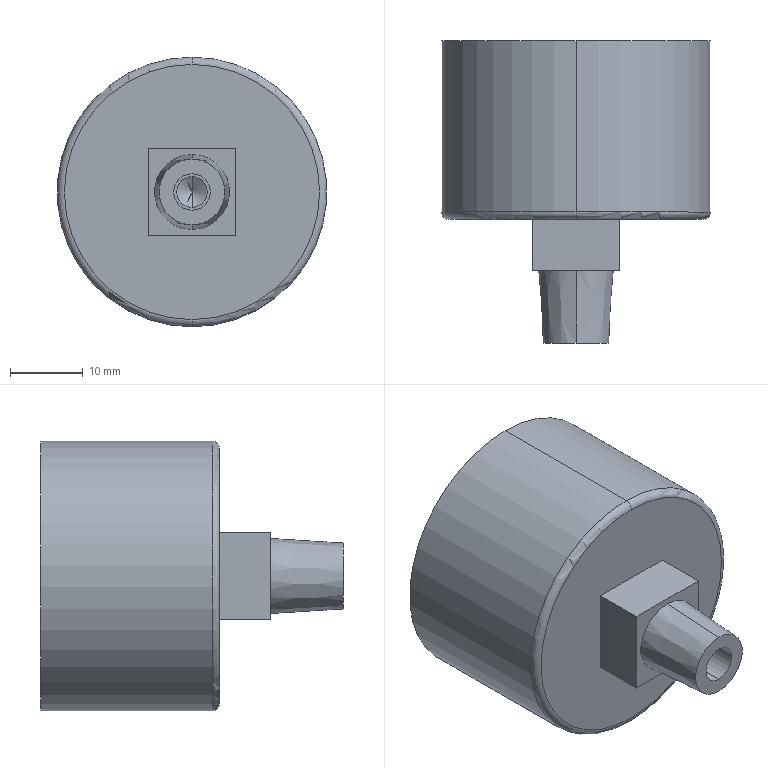Part | STEP file | VBA22A-03GN_G36-10-N01 | 1 solid | 21 faces | box 37 x 41.5 x 37 mm | volume 27826 mm3 | plane 9 | cylinder 6 | cone 4 | torus 2 | commonest cylinder face diameters 4.2 x2 5 x2 37 x2
STEP:
#1=CARTESIAN_POINT('',(0.,0.,0.));
#2=DIRECTION('',(0.,0.,1.));
#3=DIRECTION('',(1.,0.,0.));
#4=AXIS2_PLACEMENT_3D('',#1,#2,#3);
#5=CARTESIAN_POINT('',(0.,12.4,2.1));
#6=VERTEX_POINT('',#5);
#7=CARTESIAN_POINT('',(0.,12.4,-2.1));
#8=VERTEX_POINT('',#7);
#9=CARTESIAN_POINT('',(0.,12.4,0.));
#10=DIRECTION('',(0.,-1.,0.));
#11=DIRECTION('',(0.,0.,-1.));
#12=AXIS2_PLACEMENT_3D('',#9,#10,#11);
#13=CIRCLE('',#12,2.1);
#14=CARTESIAN_POINT('',(0.,12.4,0.));
#15=DIRECTION('',(0.,-1.,0.));
#16=DIRECTION('',(0.,0.,-1.));
#17=AXIS2_PLACEMENT_3D('',#14,#15,#16);
#18=CONICAL_SURFACE('',#17,2.1,1.03);
#19=CARTESIAN_POINT('',(0.,0.));
#20=DIRECTION('',(1.,0.));
#21=VECTOR('',#20,1.);
#22=LINE('',#19,#21);
#23=(GEOMETRIC_REPRESENTATION_CONTEXT(2)PARAMETRIC_REPRESENTATION_CONTEXT()REPRESENTATION_CONTEXT('',''));
#24=DEFINITIONAL_REPRESENTATION('',(#22),#23);
#25=PCURVE('',#18,#24);
#26=CARTESIAN_POINT('',(0.,0.,0.));
#27=DIRECTION('',(0.,-1.,0.));
#28=DIRECTION('',(0.,0.,-1.));
#29=AXIS2_PLACEMENT_3D('',#26,#27,#28);
#30=CYLINDRICAL_SURFACE('',#29,2.1);
#31=CARTESIAN_POINT('',(0.,-12.4));
#32=DIRECTION('',(1.,0.));
#33=VECTOR('',#32,1.);
#34=LINE('',#31,#33);
#35=(GEOMETRIC_REPRESENTATION_CONTEXT(2)PARAMETRIC_REPRESENTATION_CONTEXT()REPRESENTATION_CONTEXT('',''));
#36=DEFINITIONAL_REPRESENTATION('',(#34),#35);
#37=PCURVE('',#30,#36);
#38=SURFACE_CURVE('',#13,(#25,#37),.PCURVE_S1.);
#39=EDGE_CURVE('',#6,#8,#38,.T.);
#40=ORIENTED_EDGE('',*,*,#39,.F.);
#41=CARTESIAN_POINT('',(0.,13.662,0.));
#42=VERTEX_POINT('',#41);
#43=CARTESIAN_POINT('',(0.,12.4,2.1));
#44=DIRECTION('',(0.,-0.515,0.8572));
#45=VECTOR('',#44,1.);
#46=LINE('',#43,#45);
#47=CARTESIAN_POINT('',(3.142,0.));
#48=DIRECTION('',(0.,1.));
#49=VECTOR('',#48,1.);
#50=LINE('',#47,#49);
#51=(GEOMETRIC_REPRESENTATION_CONTEXT(2)PARAMETRIC_REPRESENTATION_CONTEXT()REPRESENTATION_CONTEXT('',''));
#52=DEFINITIONAL_REPRESENTATION('',(#50),#51);
#53=PCURVE('',#18,#52);
#54=CARTESIAN_POINT('',(0.,12.4,0.));
#55=DIRECTION('',(0.,-1.,0.));
#56=DIRECTION('',(0.,0.,-1.));
#57=AXIS2_PLACEMENT_3D('',#54,#55,#56);
#58=CONICAL_SURFACE('',#57,2.1,1.03);
#59=CARTESIAN_POINT('',(3.142,0.));
#60=DIRECTION('',(0.,1.));
#61=VECTOR('',#60,1.);
#62=LINE('',#59,#61);
#63=(GEOMETRIC_REPRESENTATION_CONTEXT(2)PARAMETRIC_REPRESENTATION_CONTEXT()REPRESENTATION_CONTEXT('',''));
#64=DEFINITIONAL_REPRESENTATION('',(#62),#63);
#65=PCURVE('',#58,#64);
#66=SURFACE_CURVE('',#46,(#53,#65),.PCURVE_S1.);
#67=EDGE_CURVE('',#42,#6,#66,.T.);
#68=ORIENTED_EDGE('',*,*,#67,.F.);
#69=CARTESIAN_POINT('',(0.,12.4,-2.1));
#70=DIRECTION('',(0.,-0.515,-0.8572));
#71=VECTOR('',#70,1.);
#72=LINE('',#69,#71);
#73=CARTESIAN_POINT('',(6.283,0.));
#74=DIRECTION('',(0.,1.));
#75=VECTOR('',#74,1.);
#76=LINE('',#73,#75);
#77=(GEOMETRIC_REPRESENTATION_CONTEXT(2)PARAMETRIC_REPRESENTATION_CONTEXT()REPRESENTATION_CONTEXT('',''));
#78=DEFINITIONAL_REPRESENTATION('',(#76),#77);
#79=PCURVE('',#18,#78);
#80=CARTESIAN_POINT('',(0.,0.));
#81=DIRECTION('',(0.,1.));
#82=VECTOR('',#81,1.);
#83=LINE('',#80,#82);
#84=(GEOMETRIC_REPRESENTATION_CONTEXT(2)PARAMETRIC_REPRESENTATION_CONTEXT()REPRESENTATION_CONTEXT('',''));
#85=DEFINITIONAL_REPRESENTATION('',(#83),#84);
#86=PCURVE('',#58,#85);
#87=SURFACE_CURVE('',#72,(#79,#86),.PCURVE_S1.);
#88=EDGE_CURVE('',#42,#8,#87,.T.);
#89=ORIENTED_EDGE('',*,*,#88,.T.);
#90=EDGE_LOOP('',(#40,#68,#89));
#91=FACE_BOUND('',#90,.F.);
#92=ADVANCED_FACE('',(#91),#18,.F.);
#93=CARTESIAN_POINT('',(0.,10.,-2.1));
#94=VERTEX_POINT('',#93);
#95=CARTESIAN_POINT('',(0.,0.,-2.1));
#96=DIRECTION('',(0.,-1.,0.));
#97=VECTOR('',#96,1.);
#98=LINE('',#95,#97);
#99=CARTESIAN_POINT('',(6.283,0.));
#100=DIRECTION('',(0.,1.));
#101=VECTOR('',#100,1.);
#102=LINE('',#99,#101);
#103=(GEOMETRIC_REPRESENTATION_CONTEXT(2)PARAMETRIC_REPRESENTATION_CONTEXT()REPRESENTATION_CONTEXT('',''));
#104=DEFINITIONAL_REPRESENTATION('',(#102),#103);
#105=PCURVE('',#30,#104);
#106=CARTESIAN_POINT('',(0.,0.,0.));
#107=DIRECTION('',(0.,-1.,0.));
#108=DIRECTION('',(0.,0.,-1.));
#109=AXIS2_PLACEMENT_3D('',#106,#107,#108);
#110=CYLINDRICAL_SURFACE('',#109,2.1);
#111=CARTESIAN_POINT('',(0.,0.));
#112=DIRECTION('',(0.,1.));
#113=VECTOR('',#112,1.);
#114=LINE('',#111,#113);
#115=(GEOMETRIC_REPRESENTATION_CONTEXT(2)PARAMETRIC_REPRESENTATION_CONTEXT()REPRESENTATION_CONTEXT('',''));
#116=DEFINITIONAL_REPRESENTATION('',(#114),#115);
#117=PCURVE('',#110,#116);
#118=SURFACE_CURVE('',#98,(#105,#117),.PCURVE_S1.);
#119=EDGE_CURVE('',#8,#94,#118,.T.);
#120=ORIENTED_EDGE('',*,*,#119,.T.);
#121=CARTESIAN_POINT('',(0.,10.,2.1));
#122=VERTEX_POINT('',#121);
#123=CARTESIAN_POINT('',(0.,10.,0.));
#124=DIRECTION('',(0.,-1.,0.));
#125=DIRECTION('',(0.,0.,-1.));
#126=AXIS2_PLACEMENT_3D('',#123,#124,#125);
#127=CIRCLE('',#126,2.1);
#128=CARTESIAN_POINT('',(0.,-10.));
#129=DIRECTION('',(1.,0.));
#130=VECTOR('',#129,1.);
#131=LINE('',#128,#130);
#132=(GEOMETRIC_REPRESENTATION_CONTEXT(2)PARAMETRIC_REPRESENTATION_CONTEXT()REPRESENTATION_CONTEXT('',''));
#133=DEFINITIONAL_REPRESENTATION('',(#131),#132);
#134=PCURVE('',#30,#133);
#135=CARTESIAN_POINT('',(2.1,10.,0.));
#136=DIRECTION('',(0.,1.,0.));
#137=DIRECTION('',(0.,0.,1.));
#138=AXIS2_PLACEMENT_3D('',#135,#136,#137);
#139=PLANE('',#138);
#140=CARTESIAN_POINT('',(-2.1,-2.1));
#141=CARTESIAN_POINT('',(-2.1,1.537));
#142=CARTESIAN_POINT('',(1.05,-0.2813));
#143=CARTESIAN_POINT('',(4.2,-2.1));
#144=CARTESIAN_POINT('',(1.05,-3.919));
#145=CARTESIAN_POINT('',(-2.1,-5.737));
#146=CARTESIAN_POINT('',(-2.1,-2.1));
#147=(BOUNDED_CURVE()B_SPLINE_CURVE(2,(#140,#141,#142,#143,#144,#145,#146),.UNSPECIFIED.,.T.,.F.)B_SPLINE_CURVE_WITH_KNOTS((1,2,2,2,2,1),(-2.094,0.,2.094,4.189,6.283,8.378),.UNSPECIFIED.)CURVE()GEOMETRIC_REPRESENTATION_ITEM()RATIONAL_B_SPLINE_CURVE((1.,0.5,1.,0.5,1.,0.5,1.))REPRESENTATION_ITEM(''));
#148=(GEOMETRIC_REPRESENTATION_CONTEXT(2)PARAMETRIC_REPRESENTATION_CONTEXT()REPRESENTATION_CONTEXT('',''));
#149=DEFINITIONAL_REPRESENTATION('',(#147),#148);
#150=PCURVE('',#139,#149);
#151=SURFACE_CURVE('',#127,(#134,#150),.PCURVE_S1.);
#152=EDGE_CURVE('',#122,#94,#151,.T.);
#153=ORIENTED_EDGE('',*,*,#152,.F.);
#154=CARTESIAN_POINT('',(0.,0.,2.1));
#155=DIRECTION('',(0.,-1.,0.));
#156=VECTOR('',#155,1.);
#157=LINE('',#154,#156);
#158=CARTESIAN_POINT('',(3.142,0.));
#159=DIRECTION('',(0.,1.));
#160=VECTOR('',#159,1.);
#161=LINE('',#158,#160);
#162=(GEOMETRIC_REPRESENTATION_CONTEXT(2)PARAMETRIC_REPRESENTATION_CONTEXT()REPRESENTATION_CONTEXT('',''));
#163=DEFINITIONAL_REPRESENTATION('',(#161),#162);
#164=PCURVE('',#30,#163);
#165=CARTESIAN_POINT('',(3.142,0.));
#166=DIRECTION('',(0.,1.));
#167=VECTOR('',#166,1.);
#168=LINE('',#165,#167);
#169=(GEOMETRIC_REPRESENTATION_CONTEXT(2)PARAMETRIC_REPRESENTATION_CONTEXT()REPRESENTATION_CONTEXT('',''));
#170=DEFINITIONAL_REPRESENTATION('',(#168),#169);
#171=PCURVE('',#110,#170);
#172=SURFACE_CURVE('',#157,(#164,#171),.PCURVE_S1.);
#173=EDGE_CURVE('',#6,#122,#172,.T.);
#174=ORIENTED_EDGE('',*,*,#173,.F.);
#175=ORIENTED_EDGE('',*,*,#39,.T.);
#176=EDGE_LOOP('',(#120,#153,#174,#175));
#177=FACE_BOUND('',#176,.F.);
#178=ADVANCED_FACE('',(#177),#30,.F.);
#179=CARTESIAN_POINT('',(0.,10.,-2.5));
#180=VERTEX_POINT('',#179);
#181=CARTESIAN_POINT('',(0.,0.,-2.5));
#182=VERTEX_POINT('',#181);
#183=CARTESIAN_POINT('',(0.,0.,-2.5));
#184=DIRECTION('',(0.,-1.,0.));
#185=VECTOR('',#184,1.);
#186=LINE('',#183,#185);
#187=CARTESIAN_POINT('',(0.,0.,0.));
#188=DIRECTION('',(0.,-1.,0.));
#189=DIRECTION('',(0.,0.,-1.));
#190=AXIS2_PLACEMENT_3D('',#187,#188,#189);
#191=CYLINDRICAL_SURFACE('',#190,2.5);
#192=CARTESIAN_POINT('',(6.283,0.));
#193=DIRECTION('',(0.,1.));
#194=VECTOR('',#193,1.);
#195=LINE('',#192,#194);
#196=(GEOMETRIC_REPRESENTATION_CONTEXT(2)PARAMETRIC_REPRESENTATION_CONTEXT()REPRESENTATION_CONTEXT('',''));
#197=DEFINITIONAL_REPRESENTATION('',(#195),#196);
#198=PCURVE('',#191,#197);
#199=CARTESIAN_POINT('',(0.,0.,0.));
#200=DIRECTION('',(0.,-1.,0.));
#201=DIRECTION('',(0.,0.,-1.));
#202=AXIS2_PLACEMENT_3D('',#199,#200,#201);
#203=CYLINDRICAL_SURFACE('',#202,2.5);
#204=CARTESIAN_POINT('',(0.,0.));
#205=DIRECTION('',(0.,1.));
#206=VECTOR('',#205,1.);
#207=LINE('',#204,#206);
#208=(GEOMETRIC_REPRESENTATION_CONTEXT(2)PARAMETRIC_REPRESENTATION_CONTEXT()REPRESENTATION_CONTEXT('',''));
#209=DEFINITIONAL_REPRESENTATION('',(#207),#208);
#210=PCURVE('',#203,#209);
#211=SURFACE_CURVE('',#186,(#198,#210),.PCURVE_S1.);
#212=EDGE_CURVE('',#180,#182,#211,.T.);
#213=ORIENTED_EDGE('',*,*,#212,.T.);
#214=CARTESIAN_POINT('',(0.,0.,2.5));
#215=VERTEX_POINT('',#214);
#216=CARTESIAN_POINT('',(0.,0.,0.));
#217=DIRECTION('',(0.,-1.,0.));
#218=DIRECTION('',(0.,0.,-1.));
#219=AXIS2_PLACEMENT_3D('',#216,#217,#218);
#220=CIRCLE('',#219,2.5);
#221=CARTESIAN_POINT('',(0.,0.));
#222=DIRECTION('',(1.,0.));
#223=VECTOR('',#222,1.);
#224=LINE('',#221,#223);
#225=(GEOMETRIC_REPRESENTATION_CONTEXT(2)PARAMETRIC_REPRESENTATION_CONTEXT()REPRESENTATION_CONTEXT('',''));
#226=DEFINITIONAL_REPRESENTATION('',(#224),#225);
#227=PCURVE('',#191,#226);
#228=CARTESIAN_POINT('',(0.,0.,0.));
#229=DIRECTION('',(0.,-1.,0.));
#230=DIRECTION('',(0.,0.,-1.));
#231=AXIS2_PLACEMENT_3D('',#228,#229,#230);
#232=PLANE('',#231);
#233=CARTESIAN_POINT('',(0.,0.));
#234=DIRECTION('',(1.,0.));
#235=AXIS2_PLACEMENT_2D('',#233,#234);
#236=CIRCLE('',#235,2.5);
#237=(GEOMETRIC_REPRESENTATION_CONTEXT(2)PARAMETRIC_REPRESENTATION_CONTEXT()REPRESENTATION_CONTEXT('',''));
#238=DEFINITIONAL_REPRESENTATION('',(#236),#237);
#239=PCURVE('',#232,#238);
#240=SURFACE_CURVE('',#220,(#227,#239),.PCURVE_S1.);
#241=EDGE_CURVE('',#215,#182,#240,.T.);
#242=ORIENTED_EDGE('',*,*,#241,.F.);
#243=CARTESIAN_POINT('',(0.,10.,2.5));
#244=VERTEX_POINT('',#243);
#245=CARTESIAN_POINT('',(0.,0.,2.5));
#246=DIRECTION('',(0.,-1.,0.));
#247=VECTOR('',#246,1.);
#248=LINE('',#245,#247);
#249=CARTESIAN_POINT('',(3.142,0.));
#250=DIRECTION('',(0.,1.));
#251=VECTOR('',#250,1.);
#252=LINE('',#249,#251);
#253=(GEOMETRIC_REPRESENTATION_CONTEXT(2)PARAMETRIC_REPRESENTATION_CONTEXT()REPRESENTATION_CONTEXT('',''));
#254=DEFINITIONAL_REPRESENTATION('',(#252),#253);
#255=PCURVE('',#191,#254);
#256=CARTESIAN_POINT('',(3.142,0.));
#257=DIRECTION('',(0.,1.));
#258=VECTOR('',#257,1.);
#259=LINE('',#256,#258);
#260=(GEOMETRIC_REPRESENTATION_CONTEXT(2)PARAMETRIC_REPRESENTATION_CONTEXT()REPRESENTATION_CONTEXT('',''));
#261=DEFINITIONAL_REPRESENTATION('',(#259),#260);
#262=PCURVE('',#203,#261);
#263=SURFACE_CURVE('',#248,(#255,#262),.PCURVE_S1.);
#264=EDGE_CURVE('',#244,#215,#263,.T.);
#265=ORIENTED_EDGE('',*,*,#264,.F.);
#266=CARTESIAN_POINT('',(0.,10.,0.));
#267=DIRECTION('',(0.,-1.,0.));
#268=DIRECTION('',(0.,0.,-1.));
#269=AXIS2_PLACEMENT_3D('',#266,#267,#268);
#270=CIRCLE('',#269,2.5);
#271=CARTESIAN_POINT('',(0.,-10.));
#272=DIRECTION('',(1.,0.));
#273=VECTOR('',#272,1.);
#274=LINE('',#271,#273);
#275=(GEOMETRIC_REPRESENTATION_CONTEXT(2)PARAMETRIC_REPRESENTATION_CONTEXT()REPRESENTATION_CONTEXT('',''));
#276=DEFINITIONAL_REPRESENTATION('',(#274),#275);
#277=PCURVE('',#191,#276);
#278=CARTESIAN_POINT('',(-2.5,-2.1));
#279=CARTESIAN_POINT('',(-2.5,2.23));
#280=CARTESIAN_POINT('',(1.25,0.06506));
#281=CARTESIAN_POINT('',(5.,-2.1));
#282=CARTESIAN_POINT('',(1.25,-4.265));
#283=CARTESIAN_POINT('',(-2.5,-6.43));
#284=CARTESIAN_POINT('',(-2.5,-2.1));
#285=(BOUNDED_CURVE()B_SPLINE_CURVE(2,(#278,#279,#280,#281,#282,#283,#284),.UNSPECIFIED.,.T.,.F.)B_SPLINE_CURVE_WITH_KNOTS((1,2,2,2,2,1),(-2.094,0.,2.094,4.189,6.283,8.378),.UNSPECIFIED.)CURVE()GEOMETRIC_REPRESENTATION_ITEM()RATIONAL_B_SPLINE_CURVE((1.,0.5,1.,0.5,1.,0.5,1.))REPRESENTATION_ITEM(''));
#286=(GEOMETRIC_REPRESENTATION_CONTEXT(2)PARAMETRIC_REPRESENTATION_CONTEXT()REPRESENTATION_CONTEXT('',''));
#287=DEFINITIONAL_REPRESENTATION('',(#285),#286);
#288=PCURVE('',#139,#287);
#289=SURFACE_CURVE('',#270,(#277,#288),.PCURVE_S1.);
#290=EDGE_CURVE('',#244,#180,#289,.T.);
#291=ORIENTED_EDGE('',*,*,#290,.T.);
#292=EDGE_LOOP('',(#213,#242,#265,#291));
#293=FACE_BOUND('',#292,.F.);
#294=ADVANCED_FACE('',(#293),#191,.F.);
#295=CARTESIAN_POINT('',(0.,0.,-4.521));
#296=VERTEX_POINT('',#295);
#297=CARTESIAN_POINT('',(0.,0.,4.521));
#298=VERTEX_POINT('',#297);
#299=CARTESIAN_POINT('',(0.,0.,0.));
#300=DIRECTION('',(0.,-1.,0.));
#301=DIRECTION('',(0.,0.,-1.));
#302=AXIS2_PLACEMENT_3D('',#299,#300,#301);
#303=CIRCLE('',#302,4.521);
#304=CARTESIAN_POINT('',(0.,0.,0.));
#305=DIRECTION('',(0.,1.,0.));
#306=DIRECTION('',(0.,0.,1.));
#307=AXIS2_PLACEMENT_3D('',#304,#305,#306);
#308=CONICAL_SURFACE('',#307,4.521,0.06283);
#309=CARTESIAN_POINT('',(3.142,0.));
#310=DIRECTION('',(-1.,0.));
#311=VECTOR('',#310,1.);
#312=LINE('',#309,#311);
#313=(GEOMETRIC_REPRESENTATION_CONTEXT(2)PARAMETRIC_REPRESENTATION_CONTEXT()REPRESENTATION_CONTEXT('',''));
#314=DEFINITIONAL_REPRESENTATION('',(#312),#313);
#315=PCURVE('',#308,#314);
#316=CARTESIAN_POINT('',(0.,0.));
#317=DIRECTION('',(1.,0.));
#318=AXIS2_PLACEMENT_2D('',#316,#317);
#319=CIRCLE('',#318,4.521);
#320=(GEOMETRIC_REPRESENTATION_CONTEXT(2)PARAMETRIC_REPRESENTATION_CONTEXT()REPRESENTATION_CONTEXT('',''));
#321=DEFINITIONAL_REPRESENTATION('',(#319),#320);
#322=PCURVE('',#232,#321);
#323=SURFACE_CURVE('',#303,(#315,#322),.PCURVE_S1.);
#324=EDGE_CURVE('',#296,#298,#323,.T.);
#325=ORIENTED_EDGE('',*,*,#324,.F.);
#326=CARTESIAN_POINT('',(0.,10.,-5.15));
#327=VERTEX_POINT('',#326);
#328=CARTESIAN_POINT('',(0.,0.,-4.521));
#329=DIRECTION('',(0.,0.998,-0.06279));
#330=VECTOR('',#329,1.);
#331=LINE('',#328,#330);
#332=CARTESIAN_POINT('',(3.142,0.));
#333=DIRECTION('',(0.,1.));
#334=VECTOR('',#333,1.);
#335=LINE('',#332,#334);
#336=(GEOMETRIC_REPRESENTATION_CONTEXT(2)PARAMETRIC_REPRESENTATION_CONTEXT()REPRESENTATION_CONTEXT('',''));
#337=DEFINITIONAL_REPRESENTATION('',(#335),#336);
#338=PCURVE('',#308,#337);
#339=CARTESIAN_POINT('',(0.,0.,0.));
#340=DIRECTION('',(0.,1.,0.));
#341=DIRECTION('',(0.,0.,1.));
#342=AXIS2_PLACEMENT_3D('',#339,#340,#341);
#343=CONICAL_SURFACE('',#342,4.521,0.06283);
#344=CARTESIAN_POINT('',(3.142,0.));
#345=DIRECTION('',(0.,1.));
#346=VECTOR('',#345,1.);
#347=LINE('',#344,#346);
#348=(GEOMETRIC_REPRESENTATION_CONTEXT(2)PARAMETRIC_REPRESENTATION_CONTEXT()REPRESENTATION_CONTEXT('',''));
#349=DEFINITIONAL_REPRESENTATION('',(#347),#348);
#350=PCURVE('',#343,#349);
#351=SURFACE_CURVE('',#331,(#338,#350),.PCURVE_S1.);
#352=EDGE_CURVE('',#296,#327,#351,.T.);
#353=ORIENTED_EDGE('',*,*,#352,.T.);
#354=CARTESIAN_POINT('',(0.,10.,5.15));
#355=VERTEX_POINT('',#354);
#356=CARTESIAN_POINT('',(0.,10.,0.));
#357=DIRECTION('',(0.,-1.,0.));
#358=DIRECTION('',(0.,0.,1.));
#359=AXIS2_PLACEMENT_3D('',#356,#357,#358);
#360=CIRCLE('',#359,5.15);
#361=CARTESIAN_POINT('',(6.283,10.));
#362=DIRECTION('',(-1.,0.));
#363=VECTOR('',#362,1.);
#364=LINE('',#361,#363);
#365=(GEOMETRIC_REPRESENTATION_CONTEXT(2)PARAMETRIC_REPRESENTATION_CONTEXT()REPRESENTATION_CONTEXT('',''));
#366=DEFINITIONAL_REPRESENTATION('',(#364),#365);
#367=PCURVE('',#308,#366);
#368=CARTESIAN_POINT('',(-6.,10.,6.));
#369=DIRECTION('',(0.,1.,0.));
#370=DIRECTION('',(0.,0.,1.));
#371=AXIS2_PLACEMENT_3D('',#368,#369,#370);
#372=PLANE('',#371);
#373=CARTESIAN_POINT('',(-0.85,6.));
#374=CARTESIAN_POINT('',(-0.85,-2.92));
#375=CARTESIAN_POINT('',(-8.575,1.54));
#376=CARTESIAN_POINT('',(-16.3,6.));
#377=CARTESIAN_POINT('',(-8.575,10.46));
#378=CARTESIAN_POINT('',(-0.85,14.92));
#379=CARTESIAN_POINT('',(-0.85,6.));
#380=(BOUNDED_CURVE()B_SPLINE_CURVE(2,(#373,#374,#375,#376,#377,#378,#379),.UNSPECIFIED.,.T.,.F.)B_SPLINE_CURVE_WITH_KNOTS((1,2,2,2,2,1),(-2.094,0.,2.094,4.189,6.283,8.378),.UNSPECIFIED.)CURVE()GEOMETRIC_REPRESENTATION_ITEM()RATIONAL_B_SPLINE_CURVE((1.,0.5,1.,0.5,1.,0.5,1.))REPRESENTATION_ITEM(''));
#381=(GEOMETRIC_REPRESENTATION_CONTEXT(2)PARAMETRIC_REPRESENTATION_CONTEXT()REPRESENTATION_CONTEXT('',''));
#382=DEFINITIONAL_REPRESENTATION('',(#380),#381);
#383=PCURVE('',#372,#382);
#384=SURFACE_CURVE('',#360,(#367,#383),.PCURVE_S1.);
#385=EDGE_CURVE('',#327,#355,#384,.T.);
#386=ORIENTED_EDGE('',*,*,#385,.T.);
#387=CARTESIAN_POINT('',(0.,0.,4.521));
#388=DIRECTION('',(0.,0.998,0.06279));
#389=VECTOR('',#388,1.);
#390=LINE('',#387,#389);
#391=CARTESIAN_POINT('',(0.,0.));
#392=DIRECTION('',(0.,1.));
#393=VECTOR('',#392,1.);
#394=LINE('',#391,#393);
#395=(GEOMETRIC_REPRESENTATION_CONTEXT(2)PARAMETRIC_REPRESENTATION_CONTEXT()REPRESENTATION_CONTEXT('',''));
#396=DEFINITIONAL_REPRESENTATION('',(#394),#395);
#397=PCURVE('',#308,#396);
#398=CARTESIAN_POINT('',(6.283,0.));
#399=DIRECTION('',(0.,1.));
#400=VECTOR('',#399,1.);
#401=LINE('',#398,#400);
#402=(GEOMETRIC_REPRESENTATION_CONTEXT(2)PARAMETRIC_REPRESENTATION_CONTEXT()REPRESENTATION_CONTEXT('',''));
#403=DEFINITIONAL_REPRESENTATION('',(#401),#402);
#404=PCURVE('',#343,#403);
#405=SURFACE_CURVE('',#390,(#397,#404),.PCURVE_S1.);
#406=EDGE_CURVE('',#298,#355,#405,.T.);
#407=ORIENTED_EDGE('',*,*,#406,.F.);
#408=EDGE_LOOP('',(#325,#353,#386,#407));
#409=FACE_BOUND('',#408,.T.);
#410=ADVANCED_FACE('',(#409),#308,.T.);
#411=CARTESIAN_POINT('',(0.,41.5,-18.5));
#412=VERTEX_POINT('',#411);
#413=CARTESIAN_POINT('',(0.,41.5,18.5));
#414=VERTEX_POINT('',#413);
#415=CARTESIAN_POINT('',(0.,41.5,0.));
#416=DIRECTION('',(0.,-1.,0.));
#417=DIRECTION('',(0.,0.,-1.));
#418=AXIS2_PLACEMENT_3D('',#415,#416,#417);
#419=CIRCLE('',#418,18.5);
#420=CARTESIAN_POINT('',(0.,0.,0.));
#421=DIRECTION('',(0.,-1.,0.));
#422=DIRECTION('',(0.,0.,-1.));
#423=AXIS2_PLACEMENT_3D('',#420,#421,#422);
#424=CYLINDRICAL_SURFACE('',#423,18.5);
#425=CARTESIAN_POINT('',(0.,-41.5));
#426=DIRECTION('',(1.,0.));
#427=VECTOR('',#426,1.);
#428=LINE('',#425,#427);
#429=(GEOMETRIC_REPRESENTATION_CONTEXT(2)PARAMETRIC_REPRESENTATION_CONTEXT()REPRESENTATION_CONTEXT('',''));
#430=DEFINITIONAL_REPRESENTATION('',(#428),#429);
#431=PCURVE('',#424,#430);
#432=CARTESIAN_POINT('',(0.,41.5,-18.5));
#433=DIRECTION('',(0.,1.,0.));
#434=DIRECTION('',(0.,0.,1.));
#435=AXIS2_PLACEMENT_3D('',#432,#433,#434);
#436=PLANE('',#435);
#437=CARTESIAN_POINT('',(0.,0.));
#438=CARTESIAN_POINT('',(0.,32.043));
#439=CARTESIAN_POINT('',(27.75,16.021));
#440=CARTESIAN_POINT('',(55.5,0.));
#441=CARTESIAN_POINT('',(27.75,-16.021));
#442=CARTESIAN_POINT('',(0.,-32.043));
#443=CARTESIAN_POINT('',(0.,0.));
#444=(BOUNDED_CURVE()B_SPLINE_CURVE(2,(#437,#438,#439,#440,#441,#442,#443),.UNSPECIFIED.,.T.,.F.)B_SPLINE_CURVE_WITH_KNOTS((1,2,2,2,2,1),(-2.094,0.,2.094,4.189,6.283,8.378),.UNSPECIFIED.)CURVE()GEOMETRIC_REPRESENTATION_ITEM()RATIONAL_B_SPLINE_CURVE((1.,0.5,1.,0.5,1.,0.5,1.))REPRESENTATION_ITEM(''));
#445=(GEOMETRIC_REPRESENTATION_CONTEXT(2)PARAMETRIC_REPRESENTATION_CONTEXT()REPRESENTATION_CONTEXT('',''));
#446=DEFINITIONAL_REPRESENTATION('',(#444),#445);
#447=PCURVE('',#436,#446);
#448=SURFACE_CURVE('',#419,(#431,#447),.PCURVE_S1.);
#449=EDGE_CURVE('',#412,#414,#448,.T.);
#450=ORIENTED_EDGE('',*,*,#449,.T.);
#451=CARTESIAN_POINT('',(0.,18.,18.5));
#452=VERTEX_POINT('',#451);
#453=CARTESIAN_POINT('',(0.,0.,18.5));
#454=DIRECTION('',(0.,-1.,0.));
#455=VECTOR('',#454,1.);
#456=LINE('',#453,#455);
#457=CARTESIAN_POINT('',(3.142,0.));
#458=DIRECTION('',(0.,1.));
#459=VECTOR('',#458,1.);
#460=LINE('',#457,#459);
#461=(GEOMETRIC_REPRESENTATION_CONTEXT(2)PARAMETRIC_REPRESENTATION_CONTEXT()REPRESENTATION_CONTEXT('',''));
#462=DEFINITIONAL_REPRESENTATION('',(#460),#461);
#463=PCURVE('',#424,#462);
#464=CARTESIAN_POINT('',(0.,0.,0.));
#465=DIRECTION('',(0.,-1.,0.));
#466=DIRECTION('',(0.,0.,-1.));
#467=AXIS2_PLACEMENT_3D('',#464,#465,#466);
#468=CYLINDRICAL_SURFACE('',#467,18.5);
#469=CARTESIAN_POINT('',(3.142,0.));
#470=DIRECTION('',(0.,1.));
#471=VECTOR('',#470,1.);
#472=LINE('',#469,#471);
#473=(GEOMETRIC_REPRESENTATION_CONTEXT(2)PARAMETRIC_REPRESENTATION_CONTEXT()REPRESENTATION_CONTEXT('',''));
#474=DEFINITIONAL_REPRESENTATION('',(#472),#473);
#475=PCURVE('',#468,#474);
#476=SURFACE_CURVE('',#456,(#463,#475),.PCURVE_S1.);
#477=EDGE_CURVE('',#414,#452,#476,.T.);
#478=ORIENTED_EDGE('',*,*,#477,.T.);
#479=CARTESIAN_POINT('',(0.,18.,-18.5));
#480=VERTEX_POINT('',#479);
#481=CARTESIAN_POINT('',(0.,18.,0.));
#482=DIRECTION('',(0.,-1.,0.));
#483=DIRECTION('',(0.,0.,-1.));
#484=AXIS2_PLACEMENT_3D('',#481,#482,#483);
#485=CIRCLE('',#484,18.5);
#486=CARTESIAN_POINT('',(0.,-18.));
#487=DIRECTION('',(1.,0.));
#488=VECTOR('',#487,1.);
#489=LINE('',#486,#488);
#490=(GEOMETRIC_REPRESENTATION_CONTEXT(2)PARAMETRIC_REPRESENTATION_CONTEXT()REPRESENTATION_CONTEXT('',''));
#491=DEFINITIONAL_REPRESENTATION('',(#489),#490);
#492=PCURVE('',#424,#491);
#493=CARTESIAN_POINT('',(0.,18.,0.));
#494=DIRECTION('',(0.,-1.,0.));
#495=DIRECTION('',(0.,0.,-1.));
#496=AXIS2_PLACEMENT_3D('',#493,#494,#495);
#497=TOROIDAL_SURFACE('',#496,17.5,1.);
#498=CARTESIAN_POINT('',(0.,0.));
#499=DIRECTION('',(1.,0.));
#500=VECTOR('',#499,1.);
#501=LINE('',#498,#500);
#502=(GEOMETRIC_REPRESENTATION_CONTEXT(2)PARAMETRIC_REPRESENTATION_CONTEXT()REPRESENTATION_CONTEXT('',''));
#503=DEFINITIONAL_REPRESENTATION('',(#501),#502);
#504=PCURVE('',#497,#503);
#505=SURFACE_CURVE('',#485,(#492,#504),.PCURVE_S1.);
#506=EDGE_CURVE('',#480,#452,#505,.T.);
#507=ORIENTED_EDGE('',*,*,#506,.F.);
#508=CARTESIAN_POINT('',(0.,0.,-18.5));
#509=DIRECTION('',(0.,-1.,0.));
#510=VECTOR('',#509,1.);
#511=LINE('',#508,#510);
#512=CARTESIAN_POINT('',(0.,0.));
#513=DIRECTION('',(0.,1.));
#514=VECTOR('',#513,1.);
#515=LINE('',#512,#514);
#516=(GEOMETRIC_REPRESENTATION_CONTEXT(2)PARAMETRIC_REPRESENTATION_CONTEXT()REPRESENTATION_CONTEXT('',''));
#517=DEFINITIONAL_REPRESENTATION('',(#515),#516);
#518=PCURVE('',#424,#517);
#519=CARTESIAN_POINT('',(6.283,0.));
#520=DIRECTION('',(0.,1.));
#521=VECTOR('',#520,1.);
#522=LINE('',#519,#521);
#523=(GEOMETRIC_REPRESENTATION_CONTEXT(2)PARAMETRIC_REPRESENTATION_CONTEXT()REPRESENTATION_CONTEXT('',''));
#524=DEFINITIONAL_REPRESENTATION('',(#522),#523);
#525=PCURVE('',#468,#524);
#526=SURFACE_CURVE('',#511,(#518,#525),.PCURVE_S1.);
#527=EDGE_CURVE('',#412,#480,#526,.T.);
#528=ORIENTED_EDGE('',*,*,#527,.F.);
#529=EDGE_LOOP('',(#450,#478,#507,#528));
#530=FACE_BOUND('',#529,.T.);
#531=ADVANCED_FACE('',(#530),#424,.T.);
#532=ORIENTED_EDGE('',*,*,#506,.T.);
#533=CARTESIAN_POINT('',(0.,17.,17.5));
#534=VERTEX_POINT('',#533);
#535=CARTESIAN_POINT('',(0.,18.,17.5));
#536=DIRECTION('',(1.,0.,0.));
#537=DIRECTION('',(0.,0.,-1.));
#538=AXIS2_PLACEMENT_3D('',#535,#536,#537);
#539=CIRCLE('',#538,1.);
#540=CARTESIAN_POINT('',(3.142,-3.142));
#541=DIRECTION('',(0.,1.));
#542=VECTOR('',#541,1.);
#543=LINE('',#540,#542);
#544=(GEOMETRIC_REPRESENTATION_CONTEXT(2)PARAMETRIC_REPRESENTATION_CONTEXT()REPRESENTATION_CONTEXT('',''));
#545=DEFINITIONAL_REPRESENTATION('',(#543),#544);
#546=PCURVE('',#497,#545);
#547=CARTESIAN_POINT('',(0.,18.,0.));
#548=DIRECTION('',(0.,-1.,0.));
#549=DIRECTION('',(0.,0.,-1.));
#550=AXIS2_PLACEMENT_3D('',#547,#548,#549);
#551=TOROIDAL_SURFACE('',#550,17.5,1.);
#552=CARTESIAN_POINT('',(3.142,-3.142));
#553=DIRECTION('',(0.,1.));
#554=VECTOR('',#553,1.);
#555=LINE('',#552,#554);
#556=(GEOMETRIC_REPRESENTATION_CONTEXT(2)PARAMETRIC_REPRESENTATION_CONTEXT()REPRESENTATION_CONTEXT('',''));
#557=DEFINITIONAL_REPRESENTATION('',(#555),#556);
#558=PCURVE('',#551,#557);
#559=SURFACE_CURVE('',#539,(#546,#558),.PCURVE_S1.);
#560=EDGE_CURVE('',#452,#534,#559,.T.);
#561=ORIENTED_EDGE('',*,*,#560,.T.);
#562=CARTESIAN_POINT('',(0.,17.,-17.5));
#563=VERTEX_POINT('',#562);
#564=CARTESIAN_POINT('',(0.,17.,0.));
#565=DIRECTION('',(0.,-1.,0.));
#566=DIRECTION('',(0.,0.,-1.));
#567=AXIS2_PLACEMENT_3D('',#564,#565,#566);
#568=CIRCLE('',#567,17.5);
#569=CARTESIAN_POINT('',(0.,1.571));
#570=DIRECTION('',(1.,0.));
#571=VECTOR('',#570,1.);
#572=LINE('',#569,#571);
#573=(GEOMETRIC_REPRESENTATION_CONTEXT(2)PARAMETRIC_REPRESENTATION_CONTEXT()REPRESENTATION_CONTEXT('',''));
#574=DEFINITIONAL_REPRESENTATION('',(#572),#573);
#575=PCURVE('',#497,#574);
#576=CARTESIAN_POINT('',(0.,17.,-5.15));
#577=DIRECTION('',(0.,-1.,0.));
#578=DIRECTION('',(0.,0.,-1.));
#579=AXIS2_PLACEMENT_3D('',#576,#577,#578);
#580=PLANE('',#579);
#581=CARTESIAN_POINT('',(-5.15,0.));
#582=DIRECTION('',(1.,0.));
#583=AXIS2_PLACEMENT_2D('',#581,#582);
#584=CIRCLE('',#583,17.5);
#585=(GEOMETRIC_REPRESENTATION_CONTEXT(2)PARAMETRIC_REPRESENTATION_CONTEXT()REPRESENTATION_CONTEXT('',''));
#586=DEFINITIONAL_REPRESENTATION('',(#584),#585);
#587=PCURVE('',#580,#586);
#588=SURFACE_CURVE('',#568,(#575,#587),.PCURVE_S1.);
#589=EDGE_CURVE('',#563,#534,#588,.T.);
#590=ORIENTED_EDGE('',*,*,#589,.F.);
#591=CARTESIAN_POINT('',(0.,18.,-17.5));
#592=DIRECTION('',(-1.,0.,0.));
#593=DIRECTION('',(0.,0.,1.));
#594=AXIS2_PLACEMENT_3D('',#591,#592,#593);
#595=CIRCLE('',#594,1.);
#596=CARTESIAN_POINT('',(0.,-3.142));
#597=DIRECTION('',(0.,1.));
#598=VECTOR('',#597,1.);
#599=LINE('',#596,#598);
#600=(GEOMETRIC_REPRESENTATION_CONTEXT(2)PARAMETRIC_REPRESENTATION_CONTEXT()REPRESENTATION_CONTEXT('',''));
#601=DEFINITIONAL_REPRESENTATION('',(#599),#600);
#602=PCURVE('',#497,#601);
#603=CARTESIAN_POINT('',(6.283,-3.142));
#604=DIRECTION('',(0.,1.));
#605=VECTOR('',#604,1.);
#606=LINE('',#603,#605);
#607=(GEOMETRIC_REPRESENTATION_CONTEXT(2)PARAMETRIC_REPRESENTATION_CONTEXT()REPRESENTATION_CONTEXT('',''));
#608=DEFINITIONAL_REPRESENTATION('',(#606),#607);
#609=PCURVE('',#551,#608);
#610=SURFACE_CURVE('',#595,(#602,#609),.PCURVE_S1.);
#611=EDGE_CURVE('',#480,#563,#610,.T.);
#612=ORIENTED_EDGE('',*,*,#611,.F.);
#613=EDGE_LOOP('',(#532,#561,#590,#612));
#614=FACE_BOUND('',#613,.T.);
#615=ADVANCED_FACE('',(#614),#497,.T.);
#616=ORIENTED_EDGE('',*,*,#589,.T.);
#617=CARTESIAN_POINT('',(0.,17.,0.));
#618=DIRECTION('',(0.,-1.,0.));
#619=DIRECTION('',(0.,0.,-1.));
#620=AXIS2_PLACEMENT_3D('',#617,#618,#619);
#621=CIRCLE('',#620,17.5);
#622=CARTESIAN_POINT('',(-5.15,0.));
#623=DIRECTION('',(1.,0.));
#624=AXIS2_PLACEMENT_2D('',#622,#623);
#625=CIRCLE('',#624,17.5);
#626=(GEOMETRIC_REPRESENTATION_CONTEXT(2)PARAMETRIC_REPRESENTATION_CONTEXT()REPRESENTATION_CONTEXT('',''));
#627=DEFINITIONAL_REPRESENTATION('',(#625),#626);
#628=PCURVE('',#580,#627);
#629=CARTESIAN_POINT('',(0.,1.571));
#630=DIRECTION('',(1.,0.));
#631=VECTOR('',#630,1.);
#632=LINE('',#629,#631);
#633=(GEOMETRIC_REPRESENTATION_CONTEXT(2)PARAMETRIC_REPRESENTATION_CONTEXT()REPRESENTATION_CONTEXT('',''));
#634=DEFINITIONAL_REPRESENTATION('',(#632),#633);
#635=PCURVE('',#551,#634);
#636=SURFACE_CURVE('',#621,(#628,#635),.PCURVE_S1.);
#637=EDGE_CURVE('',#534,#563,#636,.T.);
#638=ORIENTED_EDGE('',*,*,#637,.T.);
#639=EDGE_LOOP('',(#616,#638));
#640=FACE_BOUND('',#639,.T.);
#641=CARTESIAN_POINT('',(-6.,17.,-6.));
#642=VERTEX_POINT('',#641);
#643=CARTESIAN_POINT('',(6.,17.,-6.));
#644=VERTEX_POINT('',#643);
#645=CARTESIAN_POINT('',(-6.,17.,-6.));
#646=DIRECTION('',(1.,0.,0.));
#647=VECTOR('',#646,1.);
#648=LINE('',#645,#647);
#649=CARTESIAN_POINT('',(0.85,-6.));
#650=DIRECTION('',(0.,1.));
#651=VECTOR('',#650,1.);
#652=LINE('',#649,#651);
#653=(GEOMETRIC_REPRESENTATION_CONTEXT(2)PARAMETRIC_REPRESENTATION_CONTEXT()REPRESENTATION_CONTEXT('',''));
#654=DEFINITIONAL_REPRESENTATION('',(#652),#653);
#655=PCURVE('',#580,#654);
#656=CARTESIAN_POINT('',(-6.,10.,-6.));
#657=DIRECTION('',(0.,0.,1.));
#658=DIRECTION('',(1.,0.,0.));
#659=AXIS2_PLACEMENT_3D('',#656,#657,#658);
#660=PLANE('',#659);
#661=CARTESIAN_POINT('',(0.,7.));
#662=DIRECTION('',(1.,0.));
#663=VECTOR('',#662,1.);
#664=LINE('',#661,#663);
#665=(GEOMETRIC_REPRESENTATION_CONTEXT(2)PARAMETRIC_REPRESENTATION_CONTEXT()REPRESENTATION_CONTEXT('',''));
#666=DEFINITIONAL_REPRESENTATION('',(#664),#665);
#667=PCURVE('',#660,#666);
#668=SURFACE_CURVE('',#648,(#655,#667),.PCURVE_S1.);
#669=EDGE_CURVE('',#642,#644,#668,.T.);
#670=ORIENTED_EDGE('',*,*,#669,.F.);
#671=CARTESIAN_POINT('',(-6.,17.,6.));
#672=VERTEX_POINT('',#671);
#673=CARTESIAN_POINT('',(-6.,17.,-6.));
#674=DIRECTION('',(0.,0.,-1.));
#675=VECTOR('',#674,1.);
#676=LINE('',#673,#675);
#677=CARTESIAN_POINT('',(0.85,-6.));
#678=DIRECTION('',(1.,0.));
#679=VECTOR('',#678,1.);
#680=LINE('',#677,#679);
#681=(GEOMETRIC_REPRESENTATION_CONTEXT(2)PARAMETRIC_REPRESENTATION_CONTEXT()REPRESENTATION_CONTEXT('',''));
#682=DEFINITIONAL_REPRESENTATION('',(#680),#681);
#683=PCURVE('',#580,#682);
#684=CARTESIAN_POINT('',(-6.,10.,-6.));
#685=DIRECTION('',(1.,0.,0.));
#686=DIRECTION('',(0.,0.,-1.));
#687=AXIS2_PLACEMENT_3D('',#684,#685,#686);
#688=PLANE('',#687);
#689=CARTESIAN_POINT('',(0.,7.));
#690=DIRECTION('',(1.,0.));
#691=VECTOR('',#690,1.);
#692=LINE('',#689,#691);
#693=(GEOMETRIC_REPRESENTATION_CONTEXT(2)PARAMETRIC_REPRESENTATION_CONTEXT()REPRESENTATION_CONTEXT('',''));
#694=DEFINITIONAL_REPRESENTATION('',(#692),#693);
#695=PCURVE('',#688,#694);
#696=SURFACE_CURVE('',#676,(#683,#695),.PCURVE_S1.);
#697=EDGE_CURVE('',#672,#642,#696,.T.);
#698=ORIENTED_EDGE('',*,*,#697,.F.);
#699=CARTESIAN_POINT('',(6.,17.,6.));
#700=VERTEX_POINT('',#699);
#701=CARTESIAN_POINT('',(-6.,17.,6.));
#702=DIRECTION('',(-1.,0.,0.));
#703=VECTOR('',#702,1.);
#704=LINE('',#701,#703);
#705=CARTESIAN_POINT('',(-11.15,-6.));
#706=DIRECTION('',(0.,-1.));
#707=VECTOR('',#706,1.);
#708=LINE('',#705,#707);
#709=(GEOMETRIC_REPRESENTATION_CONTEXT(2)PARAMETRIC_REPRESENTATION_CONTEXT()REPRESENTATION_CONTEXT('',''));
#710=DEFINITIONAL_REPRESENTATION('',(#708),#709);
#711=PCURVE('',#580,#710);
#712=CARTESIAN_POINT('',(-6.,10.,6.));
#713=DIRECTION('',(0.,0.,-1.));
#714=DIRECTION('',(-1.,0.,0.));
#715=AXIS2_PLACEMENT_3D('',#712,#713,#714);
#716=PLANE('',#715);
#717=CARTESIAN_POINT('',(0.,7.));
#718=DIRECTION('',(1.,0.));
#719=VECTOR('',#718,1.);
#720=LINE('',#717,#719);
#721=(GEOMETRIC_REPRESENTATION_CONTEXT(2)PARAMETRIC_REPRESENTATION_CONTEXT()REPRESENTATION_CONTEXT('',''));
#722=DEFINITIONAL_REPRESENTATION('',(#720),#721);
#723=PCURVE('',#716,#722);
#724=SURFACE_CURVE('',#704,(#711,#723),.PCURVE_S1.);
#725=EDGE_CURVE('',#700,#672,#724,.T.);
#726=ORIENTED_EDGE('',*,*,#725,.F.);
#727=CARTESIAN_POINT('',(6.,17.,-6.));
#728=DIRECTION('',(0.,0.,1.));
#729=VECTOR('',#728,1.);
#730=LINE('',#727,#729);
#731=CARTESIAN_POINT('',(0.85,6.));
#732=DIRECTION('',(-1.,0.));
#733=VECTOR('',#732,1.);
#734=LINE('',#731,#733);
#735=(GEOMETRIC_REPRESENTATION_CONTEXT(2)PARAMETRIC_REPRESENTATION_CONTEXT()REPRESENTATION_CONTEXT('',''));
#736=DEFINITIONAL_REPRESENTATION('',(#734),#735);
#737=PCURVE('',#580,#736);
#738=CARTESIAN_POINT('',(6.,10.,-6.));
#739=DIRECTION('',(-1.,0.,0.));
#740=DIRECTION('',(0.,0.,1.));
#741=AXIS2_PLACEMENT_3D('',#738,#739,#740);
#742=PLANE('',#741);
#743=CARTESIAN_POINT('',(0.,7.));
#744=DIRECTION('',(1.,0.));
#745=VECTOR('',#744,1.);
#746=LINE('',#743,#745);
#747=(GEOMETRIC_REPRESENTATION_CONTEXT(2)PARAMETRIC_REPRESENTATION_CONTEXT()REPRESENTATION_CONTEXT('',''));
#748=DEFINITIONAL_REPRESENTATION('',(#746),#747);
#749=PCURVE('',#742,#748);
#750=SURFACE_CURVE('',#730,(#737,#749),.PCURVE_S1.);
#751=EDGE_CURVE('',#644,#700,#750,.T.);
#752=ORIENTED_EDGE('',*,*,#751,.F.);
#753=EDGE_LOOP('',(#670,#698,#726,#752));
#754=FACE_BOUND('',#753,.T.);
#755=ADVANCED_FACE('',(#640,#754),#580,.T.);
#756=ORIENTED_EDGE('',*,*,#560,.F.);
#757=CARTESIAN_POINT('',(0.,18.,0.));
#758=DIRECTION('',(0.,-1.,0.));
#759=DIRECTION('',(0.,0.,-1.));
#760=AXIS2_PLACEMENT_3D('',#757,#758,#759);
#761=CIRCLE('',#760,18.5);
#762=CARTESIAN_POINT('',(0.,0.));
#763=DIRECTION('',(1.,0.));
#764=VECTOR('',#763,1.);
#765=LINE('',#762,#764);
#766=(GEOMETRIC_REPRESENTATION_CONTEXT(2)PARAMETRIC_REPRESENTATION_CONTEXT()REPRESENTATION_CONTEXT('',''));
#767=DEFINITIONAL_REPRESENTATION('',(#765),#766);
#768=PCURVE('',#551,#767);
#769=CARTESIAN_POINT('',(0.,-18.));
#770=DIRECTION('',(1.,0.));
#771=VECTOR('',#770,1.);
#772=LINE('',#769,#771);
#773=(GEOMETRIC_REPRESENTATION_CONTEXT(2)PARAMETRIC_REPRESENTATION_CONTEXT()REPRESENTATION_CONTEXT('',''));
#774=DEFINITIONAL_REPRESENTATION('',(#772),#773);
#775=PCURVE('',#468,#774);
#776=SURFACE_CURVE('',#761,(#768,#775),.PCURVE_S1.);
#777=EDGE_CURVE('',#452,#480,#776,.T.);
#778=ORIENTED_EDGE('',*,*,#777,.T.);
#779=ORIENTED_EDGE('',*,*,#611,.T.);
#780=ORIENTED_EDGE('',*,*,#637,.F.);
#781=EDGE_LOOP('',(#756,#778,#779,#780));
#782=FACE_BOUND('',#781,.T.);
#783=ADVANCED_FACE('',(#782),#551,.T.);
#784=ORIENTED_EDGE('',*,*,#477,.F.);
#785=CARTESIAN_POINT('',(0.,41.5,0.));
#786=DIRECTION('',(0.,-1.,0.));
#787=DIRECTION('',(0.,0.,-1.));
#788=AXIS2_PLACEMENT_3D('',#785,#786,#787);
#789=CIRCLE('',#788,18.5);
#790=CARTESIAN_POINT('',(0.,-41.5));
#791=DIRECTION('',(1.,0.));
#792=VECTOR('',#791,1.);
#793=LINE('',#790,#792);
#794=(GEOMETRIC_REPRESENTATION_CONTEXT(2)PARAMETRIC_REPRESENTATION_CONTEXT()REPRESENTATION_CONTEXT('',''));
#795=DEFINITIONAL_REPRESENTATION('',(#793),#794);
#796=PCURVE('',#468,#795);
#797=CARTESIAN_POINT('',(0.,0.));
#798=CARTESIAN_POINT('',(0.,32.043));
#799=CARTESIAN_POINT('',(27.75,16.021));
#800=CARTESIAN_POINT('',(55.5,0.));
#801=CARTESIAN_POINT('',(27.75,-16.021));
#802=CARTESIAN_POINT('',(0.,-32.043));
#803=CARTESIAN_POINT('',(0.,0.));
#804=(BOUNDED_CURVE()B_SPLINE_CURVE(2,(#797,#798,#799,#800,#801,#802,#803),.UNSPECIFIED.,.T.,.F.)B_SPLINE_CURVE_WITH_KNOTS((1,2,2,2,2,1),(-2.094,0.,2.094,4.189,6.283,8.378),.UNSPECIFIED.)CURVE()GEOMETRIC_REPRESENTATION_ITEM()RATIONAL_B_SPLINE_CURVE((1.,0.5,1.,0.5,1.,0.5,1.))REPRESENTATION_ITEM(''));
#805=(GEOMETRIC_REPRESENTATION_CONTEXT(2)PARAMETRIC_REPRESENTATION_CONTEXT()REPRESENTATION_CONTEXT('',''));
#806=DEFINITIONAL_REPRESENTATION('',(#804),#805);
#807=PCURVE('',#436,#806);
#808=SURFACE_CURVE('',#789,(#796,#807),.PCURVE_S1.);
#809=EDGE_CURVE('',#414,#412,#808,.T.);
#810=ORIENTED_EDGE('',*,*,#809,.T.);
#811=ORIENTED_EDGE('',*,*,#527,.T.);
#812=ORIENTED_EDGE('',*,*,#777,.F.);
#813=EDGE_LOOP('',(#784,#810,#811,#812));
#814=FACE_BOUND('',#813,.T.);
#815=ADVANCED_FACE('',(#814),#468,.T.);
#816=ORIENTED_EDGE('',*,*,#449,.F.);
#817=ORIENTED_EDGE('',*,*,#809,.F.);
#818=EDGE_LOOP('',(#816,#817));
#819=FACE_BOUND('',#818,.T.);
#820=ADVANCED_FACE('',(#819),#436,.T.);
#821=ORIENTED_EDGE('',*,*,#697,.T.);
#822=CARTESIAN_POINT('',(-6.,10.,-6.));
#823=VERTEX_POINT('',#822);
#824=CARTESIAN_POINT('',(-6.,10.,-6.));
#825=DIRECTION('',(0.,1.,0.));
#826=VECTOR('',#825,1.);
#827=LINE('',#824,#826);
#828=CARTESIAN_POINT('',(0.,0.));
#829=DIRECTION('',(0.,1.));
#830=VECTOR('',#829,1.);
#831=LINE('',#828,#830);
#832=(GEOMETRIC_REPRESENTATION_CONTEXT(2)PARAMETRIC_REPRESENTATION_CONTEXT()REPRESENTATION_CONTEXT('',''));
#833=DEFINITIONAL_REPRESENTATION('',(#831),#832);
#834=PCURVE('',#688,#833);
#835=CARTESIAN_POINT('',(0.,0.));
#836=DIRECTION('',(0.,1.));
#837=VECTOR('',#836,1.);
#838=LINE('',#835,#837);
#839=(GEOMETRIC_REPRESENTATION_CONTEXT(2)PARAMETRIC_REPRESENTATION_CONTEXT()REPRESENTATION_CONTEXT('',''));
#840=DEFINITIONAL_REPRESENTATION('',(#838),#839);
#841=PCURVE('',#660,#840);
#842=SURFACE_CURVE('',#827,(#834,#841),.PCURVE_S1.);
#843=EDGE_CURVE('',#823,#642,#842,.T.);
#844=ORIENTED_EDGE('',*,*,#843,.F.);
#845=CARTESIAN_POINT('',(-6.,10.,6.));
#846=VERTEX_POINT('',#845);
#847=CARTESIAN_POINT('',(-6.,10.,-6.));
#848=DIRECTION('',(0.,0.,-1.));
#849=VECTOR('',#848,1.);
#850=LINE('',#847,#849);
#851=CARTESIAN_POINT('',(0.,0.));
#852=DIRECTION('',(1.,0.));
#853=VECTOR('',#852,1.);
#854=LINE('',#851,#853);
#855=(GEOMETRIC_REPRESENTATION_CONTEXT(2)PARAMETRIC_REPRESENTATION_CONTEXT()REPRESENTATION_CONTEXT('',''));
#856=DEFINITIONAL_REPRESENTATION('',(#854),#855);
#857=PCURVE('',#688,#856);
#858=CARTESIAN_POINT('',(-12.,0.));
#859=DIRECTION('',(-1.,0.));
#860=VECTOR('',#859,1.);
#861=LINE('',#858,#860);
#862=(GEOMETRIC_REPRESENTATION_CONTEXT(2)PARAMETRIC_REPRESENTATION_CONTEXT()REPRESENTATION_CONTEXT('',''));
#863=DEFINITIONAL_REPRESENTATION('',(#861),#862);
#864=PCURVE('',#372,#863);
#865=SURFACE_CURVE('',#850,(#857,#864),.PCURVE_S1.);
#866=EDGE_CURVE('',#846,#823,#865,.T.);
#867=ORIENTED_EDGE('',*,*,#866,.F.);
#868=CARTESIAN_POINT('',(-6.,10.,6.));
#869=DIRECTION('',(0.,1.,0.));
#870=VECTOR('',#869,1.);
#871=LINE('',#868,#870);
#872=CARTESIAN_POINT('',(-12.,0.));
#873=DIRECTION('',(0.,1.));
#874=VECTOR('',#873,1.);
#875=LINE('',#872,#874);
#876=(GEOMETRIC_REPRESENTATION_CONTEXT(2)PARAMETRIC_REPRESENTATION_CONTEXT()REPRESENTATION_CONTEXT('',''));
#877=DEFINITIONAL_REPRESENTATION('',(#875),#876);
#878=PCURVE('',#688,#877);
#879=CARTESIAN_POINT('',(0.,0.));
#880=DIRECTION('',(0.,1.));
#881=VECTOR('',#880,1.);
#882=LINE('',#879,#881);
#883=(GEOMETRIC_REPRESENTATION_CONTEXT(2)PARAMETRIC_REPRESENTATION_CONTEXT()REPRESENTATION_CONTEXT('',''));
#884=DEFINITIONAL_REPRESENTATION('',(#882),#883);
#885=PCURVE('',#716,#884);
#886=SURFACE_CURVE('',#871,(#878,#885),.PCURVE_S1.);
#887=EDGE_CURVE('',#846,#672,#886,.T.);
#888=ORIENTED_EDGE('',*,*,#887,.T.);
#889=EDGE_LOOP('',(#821,#844,#867,#888));
#890=FACE_BOUND('',#889,.T.);
#891=ADVANCED_FACE('',(#890),#688,.F.);
#892=ORIENTED_EDGE('',*,*,#669,.T.);
#893=CARTESIAN_POINT('',(6.,10.,-6.));
#894=VERTEX_POINT('',#893);
#895=CARTESIAN_POINT('',(6.,10.,-6.));
#896=DIRECTION('',(0.,1.,0.));
#897=VECTOR('',#896,1.);
#898=LINE('',#895,#897);
#899=CARTESIAN_POINT('',(12.,0.));
#900=DIRECTION('',(0.,1.));
#901=VECTOR('',#900,1.);
#902=LINE('',#899,#901);
#903=(GEOMETRIC_REPRESENTATION_CONTEXT(2)PARAMETRIC_REPRESENTATION_CONTEXT()REPRESENTATION_CONTEXT('',''));
#904=DEFINITIONAL_REPRESENTATION('',(#902),#903);
#905=PCURVE('',#660,#904);
#906=CARTESIAN_POINT('',(0.,0.));
#907=DIRECTION('',(0.,1.));
#908=VECTOR('',#907,1.);
#909=LINE('',#906,#908);
#910=(GEOMETRIC_REPRESENTATION_CONTEXT(2)PARAMETRIC_REPRESENTATION_CONTEXT()REPRESENTATION_CONTEXT('',''));
#911=DEFINITIONAL_REPRESENTATION('',(#909),#910);
#912=PCURVE('',#742,#911);
#913=SURFACE_CURVE('',#898,(#905,#912),.PCURVE_S1.);
#914=EDGE_CURVE('',#894,#644,#913,.T.);
#915=ORIENTED_EDGE('',*,*,#914,.F.);
#916=CARTESIAN_POINT('',(-6.,10.,-6.));
#917=DIRECTION('',(1.,0.,0.));
#918=VECTOR('',#917,1.);
#919=LINE('',#916,#918);
#920=CARTESIAN_POINT('',(0.,0.));
#921=DIRECTION('',(1.,0.));
#922=VECTOR('',#921,1.);
#923=LINE('',#920,#922);
#924=(GEOMETRIC_REPRESENTATION_CONTEXT(2)PARAMETRIC_REPRESENTATION_CONTEXT()REPRESENTATION_CONTEXT('',''));
#925=DEFINITIONAL_REPRESENTATION('',(#923),#924);
#926=PCURVE('',#660,#925);
#927=CARTESIAN_POINT('',(-12.,0.));
#928=DIRECTION('',(0.,1.));
#929=VECTOR('',#928,1.);
#930=LINE('',#927,#929);
#931=(GEOMETRIC_REPRESENTATION_CONTEXT(2)PARAMETRIC_REPRESENTATION_CONTEXT()REPRESENTATION_CONTEXT('',''));
#932=DEFINITIONAL_REPRESENTATION('',(#930),#931);
#933=PCURVE('',#372,#932);
#934=SURFACE_CURVE('',#919,(#926,#933),.PCURVE_S1.);
#935=EDGE_CURVE('',#823,#894,#934,.T.);
#936=ORIENTED_EDGE('',*,*,#935,.F.);
#937=ORIENTED_EDGE('',*,*,#843,.T.);
#938=EDGE_LOOP('',(#892,#915,#936,#937));
#939=FACE_BOUND('',#938,.T.);
#940=ADVANCED_FACE('',(#939),#660,.F.);
#941=ORIENTED_EDGE('',*,*,#751,.T.);
#942=CARTESIAN_POINT('',(6.,10.,6.));
#943=VERTEX_POINT('',#942);
#944=CARTESIAN_POINT('',(6.,10.,6.));
#945=DIRECTION('',(0.,1.,0.));
#946=VECTOR('',#945,1.);
#947=LINE('',#944,#946);
#948=CARTESIAN_POINT('',(12.,0.));
#949=DIRECTION('',(0.,1.));
#950=VECTOR('',#949,1.);
#951=LINE('',#948,#950);
#952=(GEOMETRIC_REPRESENTATION_CONTEXT(2)PARAMETRIC_REPRESENTATION_CONTEXT()REPRESENTATION_CONTEXT('',''));
#953=DEFINITIONAL_REPRESENTATION('',(#951),#952);
#954=PCURVE('',#742,#953);
#955=CARTESIAN_POINT('',(-12.,0.));
#956=DIRECTION('',(0.,1.));
#957=VECTOR('',#956,1.);
#958=LINE('',#955,#957);
#959=(GEOMETRIC_REPRESENTATION_CONTEXT(2)PARAMETRIC_REPRESENTATION_CONTEXT()REPRESENTATION_CONTEXT('',''));
#960=DEFINITIONAL_REPRESENTATION('',(#958),#959);
#961=PCURVE('',#716,#960);
#962=SURFACE_CURVE('',#947,(#954,#961),.PCURVE_S1.);
#963=EDGE_CURVE('',#943,#700,#962,.T.);
#964=ORIENTED_EDGE('',*,*,#963,.F.);
#965=CARTESIAN_POINT('',(6.,10.,-6.));
#966=DIRECTION('',(0.,0.,1.));
#967=VECTOR('',#966,1.);
#968=LINE('',#965,#967);
#969=CARTESIAN_POINT('',(0.,0.));
#970=DIRECTION('',(1.,0.));
#971=VECTOR('',#970,1.);
#972=LINE('',#969,#971);
#973=(GEOMETRIC_REPRESENTATION_CONTEXT(2)PARAMETRIC_REPRESENTATION_CONTEXT()REPRESENTATION_CONTEXT('',''));
#974=DEFINITIONAL_REPRESENTATION('',(#972),#973);
#975=PCURVE('',#742,#974);
#976=CARTESIAN_POINT('',(-12.,12.));
#977=DIRECTION('',(1.,0.));
#978=VECTOR('',#977,1.);
#979=LINE('',#976,#978);
#980=(GEOMETRIC_REPRESENTATION_CONTEXT(2)PARAMETRIC_REPRESENTATION_CONTEXT()REPRESENTATION_CONTEXT('',''));
#981=DEFINITIONAL_REPRESENTATION('',(#979),#980);
#982=PCURVE('',#372,#981);
#983=SURFACE_CURVE('',#968,(#975,#982),.PCURVE_S1.);
#984=EDGE_CURVE('',#894,#943,#983,.T.);
#985=ORIENTED_EDGE('',*,*,#984,.F.);
#986=ORIENTED_EDGE('',*,*,#914,.T.);
#987=EDGE_LOOP('',(#941,#964,#985,#986));
#988=FACE_BOUND('',#987,.T.);
#989=ADVANCED_FACE('',(#988),#742,.F.);
#990=ORIENTED_EDGE('',*,*,#725,.T.);
#991=ORIENTED_EDGE('',*,*,#887,.F.);
#992=CARTESIAN_POINT('',(-6.,10.,6.));
#993=DIRECTION('',(-1.,0.,0.));
#994=VECTOR('',#993,1.);
#995=LINE('',#992,#994);
#996=CARTESIAN_POINT('',(0.,0.));
#997=DIRECTION('',(1.,0.));
#998=VECTOR('',#997,1.);
#999=LINE('',#996,#998);
#1000=(GEOMETRIC_REPRESENTATION_CONTEXT(2)PARAMETRIC_REPRESENTATION_CONTEXT()REPRESENTATION_CONTEXT('',''));
#1001=DEFINITIONAL_REPRESENTATION('',(#999),#1000);
#1002=PCURVE('',#716,#1001);
#1003=CARTESIAN_POINT('',(0.,0.));
#1004=DIRECTION('',(0.,-1.));
#1005=VECTOR('',#1004,1.);
#1006=LINE('',#1003,#1005);
#1007=(GEOMETRIC_REPRESENTATION_CONTEXT(2)PARAMETRIC_REPRESENTATION_CONTEXT()REPRESENTATION_CONTEXT('',''));
#1008=DEFINITIONAL_REPRESENTATION('',(#1006),#1007);
#1009=PCURVE('',#372,#1008);
#1010=SURFACE_CURVE('',#995,(#1002,#1009),.PCURVE_S1.);
#1011=EDGE_CURVE('',#943,#846,#1010,.T.);
#1012=ORIENTED_EDGE('',*,*,#1011,.F.);
#1013=ORIENTED_EDGE('',*,*,#963,.T.);
#1014=EDGE_LOOP('',(#990,#991,#1012,#1013));
#1015=FACE_BOUND('',#1014,.T.);
#1016=ADVANCED_FACE('',(#1015),#716,.F.);
#1017=CARTESIAN_POINT('',(0.,10.,0.));
#1018=DIRECTION('',(0.,-1.,0.));
#1019=DIRECTION('',(0.,0.,1.));
#1020=AXIS2_PLACEMENT_3D('',#1017,#1018,#1019);
#1021=CIRCLE('',#1020,5.15);
#1022=CARTESIAN_POINT('',(-0.85,6.));
#1023=CARTESIAN_POINT('',(-0.85,-2.92));
#1024=CARTESIAN_POINT('',(-8.575,1.54));
#1025=CARTESIAN_POINT('',(-16.3,6.));
#1026=CARTESIAN_POINT('',(-8.575,10.46));
#1027=CARTESIAN_POINT('',(-0.85,14.92));
#1028=CARTESIAN_POINT('',(-0.85,6.));
#1029=(BOUNDED_CURVE()B_SPLINE_CURVE(2,(#1022,#1023,#1024,#1025,#1026,#1027,#1028),.UNSPECIFIED.,.T.,.F.)B_SPLINE_CURVE_WITH_KNOTS((1,2,2,2,2,1),(-2.094,0.,2.094,4.189,6.283,8.378),.UNSPECIFIED.)CURVE()GEOMETRIC_REPRESENTATION_ITEM()RATIONAL_B_SPLINE_CURVE((1.,0.5,1.,0.5,1.,0.5,1.))REPRESENTATION_ITEM(''));
#1030=(GEOMETRIC_REPRESENTATION_CONTEXT(2)PARAMETRIC_REPRESENTATION_CONTEXT()REPRESENTATION_CONTEXT('',''));
#1031=DEFINITIONAL_REPRESENTATION('',(#1029),#1030);
#1032=PCURVE('',#372,#1031);
#1033=CARTESIAN_POINT('',(6.283,10.));
#1034=DIRECTION('',(-1.,0.));
#1035=VECTOR('',#1034,1.);
#1036=LINE('',#1033,#1035);
#1037=(GEOMETRIC_REPRESENTATION_CONTEXT(2)PARAMETRIC_REPRESENTATION_CONTEXT()REPRESENTATION_CONTEXT('',''));
#1038=DEFINITIONAL_REPRESENTATION('',(#1036),#1037);
#1039=PCURVE('',#343,#1038);
#1040=SURFACE_CURVE('',#1021,(#1032,#1039),.PCURVE_S1.);
#1041=EDGE_CURVE('',#355,#327,#1040,.T.);
#1042=ORIENTED_EDGE('',*,*,#1041,.F.);
#1043=ORIENTED_EDGE('',*,*,#385,.F.);
#1044=EDGE_LOOP('',(#1042,#1043));
#1045=FACE_BOUND('',#1044,.T.);
#1046=ORIENTED_EDGE('',*,*,#866,.T.);
#1047=ORIENTED_EDGE('',*,*,#935,.T.);
#1048=ORIENTED_EDGE('',*,*,#984,.T.);
#1049=ORIENTED_EDGE('',*,*,#1011,.T.);
#1050=EDGE_LOOP('',(#1046,#1047,#1048,#1049));
#1051=FACE_BOUND('',#1050,.T.);
#1052=ADVANCED_FACE('',(#1045,#1051),#372,.F.);
#1053=CARTESIAN_POINT('',(0.,0.,0.));
#1054=DIRECTION('',(0.,-1.,0.));
#1055=DIRECTION('',(0.,0.,-1.));
#1056=AXIS2_PLACEMENT_3D('',#1053,#1054,#1055);
#1057=CIRCLE('',#1056,2.5);
#1058=CARTESIAN_POINT('',(0.,0.));
#1059=DIRECTION('',(1.,0.));
#1060=AXIS2_PLACEMENT_2D('',#1058,#1059);
#1061=CIRCLE('',#1060,2.5);
#1062=(GEOMETRIC_REPRESENTATION_CONTEXT(2)PARAMETRIC_REPRESENTATION_CONTEXT()REPRESENTATION_CONTEXT('',''));
#1063=DEFINITIONAL_REPRESENTATION('',(#1061),#1062);
#1064=PCURVE('',#232,#1063);
#1065=CARTESIAN_POINT('',(0.,0.));
#1066=DIRECTION('',(1.,0.));
#1067=VECTOR('',#1066,1.);
#1068=LINE('',#1065,#1067);
#1069=(GEOMETRIC_REPRESENTATION_CONTEXT(2)PARAMETRIC_REPRESENTATION_CONTEXT()REPRESENTATION_CONTEXT('',''));
#1070=DEFINITIONAL_REPRESENTATION('',(#1068),#1069);
#1071=PCURVE('',#203,#1070);
#1072=SURFACE_CURVE('',#1057,(#1064,#1071),.PCURVE_S1.);
#1073=EDGE_CURVE('',#182,#215,#1072,.T.);
#1074=ORIENTED_EDGE('',*,*,#1073,.F.);
#1075=ORIENTED_EDGE('',*,*,#241,.F.);
#1076=EDGE_LOOP('',(#1074,#1075));
#1077=FACE_BOUND('',#1076,.T.);
#1078=CARTESIAN_POINT('',(0.,0.,0.));
#1079=DIRECTION('',(0.,-1.,0.));
#1080=DIRECTION('',(0.,0.,-1.));
#1081=AXIS2_PLACEMENT_3D('',#1078,#1079,#1080);
#1082=CIRCLE('',#1081,4.521);
#1083=CARTESIAN_POINT('',(0.,0.));
#1084=DIRECTION('',(1.,0.));
#1085=AXIS2_PLACEMENT_2D('',#1083,#1084);
#1086=CIRCLE('',#1085,4.521);
#1087=(GEOMETRIC_REPRESENTATION_CONTEXT(2)PARAMETRIC_REPRESENTATION_CONTEXT()REPRESENTATION_CONTEXT('',''));
#1088=DEFINITIONAL_REPRESENTATION('',(#1086),#1087);
#1089=PCURVE('',#232,#1088);
#1090=CARTESIAN_POINT('',(9.425,0.));
#1091=DIRECTION('',(-1.,0.));
#1092=VECTOR('',#1091,1.);
#1093=LINE('',#1090,#1092);
#1094=(GEOMETRIC_REPRESENTATION_CONTEXT(2)PARAMETRIC_REPRESENTATION_CONTEXT()REPRESENTATION_CONTEXT('',''));
#1095=DEFINITIONAL_REPRESENTATION('',(#1093),#1094);
#1096=PCURVE('',#343,#1095);
#1097=SURFACE_CURVE('',#1082,(#1089,#1096),.PCURVE_S1.);
#1098=EDGE_CURVE('',#298,#296,#1097,.T.);
#1099=ORIENTED_EDGE('',*,*,#1098,.T.);
#1100=ORIENTED_EDGE('',*,*,#324,.T.);
#1101=EDGE_LOOP('',(#1099,#1100));
#1102=FACE_BOUND('',#1101,.T.);
#1103=ADVANCED_FACE('',(#1077,#1102),#232,.T.);
#1104=ORIENTED_EDGE('',*,*,#352,.F.);
#1105=ORIENTED_EDGE('',*,*,#1098,.F.);
#1106=ORIENTED_EDGE('',*,*,#406,.T.);
#1107=ORIENTED_EDGE('',*,*,#1041,.T.);
#1108=EDGE_LOOP('',(#1104,#1105,#1106,#1107));
#1109=FACE_BOUND('',#1108,.T.);
#1110=ADVANCED_FACE('',(#1109),#343,.T.);
#1111=ORIENTED_EDGE('',*,*,#1073,.F.);
#1112=ORIENTED_EDGE('',*,*,#212,.F.);
#1113=CARTESIAN_POINT('',(0.,10.,0.));
#1114=DIRECTION('',(0.,-1.,0.));
#1115=DIRECTION('',(0.,0.,-1.));
#1116=AXIS2_PLACEMENT_3D('',#1113,#1114,#1115);
#1117=CIRCLE('',#1116,2.5);
#1118=CARTESIAN_POINT('',(0.,-10.));
#1119=DIRECTION('',(1.,0.));
#1120=VECTOR('',#1119,1.);
#1121=LINE('',#1118,#1120);
#1122=(GEOMETRIC_REPRESENTATION_CONTEXT(2)PARAMETRIC_REPRESENTATION_CONTEXT()REPRESENTATION_CONTEXT('',''));
#1123=DEFINITIONAL_REPRESENTATION('',(#1121),#1122);
#1124=PCURVE('',#203,#1123);
#1125=CARTESIAN_POINT('',(-2.5,-2.1));
#1126=CARTESIAN_POINT('',(-2.5,2.23));
#1127=CARTESIAN_POINT('',(1.25,0.06506));
#1128=CARTESIAN_POINT('',(5.,-2.1));
#1129=CARTESIAN_POINT('',(1.25,-4.265));
#1130=CARTESIAN_POINT('',(-2.5,-6.43));
#1131=CARTESIAN_POINT('',(-2.5,-2.1));
#1132=(BOUNDED_CURVE()B_SPLINE_CURVE(2,(#1125,#1126,#1127,#1128,#1129,#1130,#1131),.UNSPECIFIED.,.T.,.F.)B_SPLINE_CURVE_WITH_KNOTS((1,2,2,2,2,1),(-2.094,0.,2.094,4.189,6.283,8.378),.UNSPECIFIED.)CURVE()GEOMETRIC_REPRESENTATION_ITEM()RATIONAL_B_SPLINE_CURVE((1.,0.5,1.,0.5,1.,0.5,1.))REPRESENTATION_ITEM(''));
#1133=(GEOMETRIC_REPRESENTATION_CONTEXT(2)PARAMETRIC_REPRESENTATION_CONTEXT()REPRESENTATION_CONTEXT('',''));
#1134=DEFINITIONAL_REPRESENTATION('',(#1132),#1133);
#1135=PCURVE('',#139,#1134);
#1136=SURFACE_CURVE('',#1117,(#1124,#1135),.PCURVE_S1.);
#1137=EDGE_CURVE('',#180,#244,#1136,.T.);
#1138=ORIENTED_EDGE('',*,*,#1137,.T.);
#1139=ORIENTED_EDGE('',*,*,#264,.T.);
#1140=EDGE_LOOP('',(#1111,#1112,#1138,#1139));
#1141=FACE_BOUND('',#1140,.F.);
#1142=ADVANCED_FACE('',(#1141),#203,.F.);
#1143=CARTESIAN_POINT('',(0.,10.,0.));
#1144=DIRECTION('',(0.,-1.,0.));
#1145=DIRECTION('',(0.,0.,-1.));
#1146=AXIS2_PLACEMENT_3D('',#1143,#1144,#1145);
#1147=CIRCLE('',#1146,2.1);
#1148=CARTESIAN_POINT('',(-2.1,-2.1));
#1149=CARTESIAN_POINT('',(-2.1,1.537));
#1150=CARTESIAN_POINT('',(1.05,-0.2813));
#1151=CARTESIAN_POINT('',(4.2,-2.1));
#1152=CARTESIAN_POINT('',(1.05,-3.919));
#1153=CARTESIAN_POINT('',(-2.1,-5.737));
#1154=CARTESIAN_POINT('',(-2.1,-2.1));
#1155=(BOUNDED_CURVE()B_SPLINE_CURVE(2,(#1148,#1149,#1150,#1151,#1152,#1153,#1154),.UNSPECIFIED.,.T.,.F.)B_SPLINE_CURVE_WITH_KNOTS((1,2,2,2,2,1),(-2.094,0.,2.094,4.189,6.283,8.378),.UNSPECIFIED.)CURVE()GEOMETRIC_REPRESENTATION_ITEM()RATIONAL_B_SPLINE_CURVE((1.,0.5,1.,0.5,1.,0.5,1.))REPRESENTATION_ITEM(''));
#1156=(GEOMETRIC_REPRESENTATION_CONTEXT(2)PARAMETRIC_REPRESENTATION_CONTEXT()REPRESENTATION_CONTEXT('',''));
#1157=DEFINITIONAL_REPRESENTATION('',(#1155),#1156);
#1158=PCURVE('',#139,#1157);
#1159=CARTESIAN_POINT('',(0.,-10.));
#1160=DIRECTION('',(1.,0.));
#1161=VECTOR('',#1160,1.);
#1162=LINE('',#1159,#1161);
#1163=(GEOMETRIC_REPRESENTATION_CONTEXT(2)PARAMETRIC_REPRESENTATION_CONTEXT()REPRESENTATION_CONTEXT('',''));
#1164=DEFINITIONAL_REPRESENTATION('',(#1162),#1163);
#1165=PCURVE('',#110,#1164);
#1166=SURFACE_CURVE('',#1147,(#1158,#1165),.PCURVE_S1.);
#1167=EDGE_CURVE('',#94,#122,#1166,.T.);
#1168=ORIENTED_EDGE('',*,*,#1167,.F.);
#1169=ORIENTED_EDGE('',*,*,#152,.F.);
#1170=EDGE_LOOP('',(#1168,#1169));
#1171=FACE_BOUND('',#1170,.T.);
#1172=ORIENTED_EDGE('',*,*,#1137,.T.);
#1173=ORIENTED_EDGE('',*,*,#290,.T.);
#1174=EDGE_LOOP('',(#1172,#1173));
#1175=FACE_BOUND('',#1174,.T.);
#1176=ADVANCED_FACE('',(#1171,#1175),#139,.F.);
#1177=ORIENTED_EDGE('',*,*,#1167,.F.);
#1178=ORIENTED_EDGE('',*,*,#119,.F.);
#1179=CARTESIAN_POINT('',(0.,12.4,0.));
#1180=DIRECTION('',(0.,-1.,0.));
#1181=DIRECTION('',(0.,0.,-1.));
#1182=AXIS2_PLACEMENT_3D('',#1179,#1180,#1181);
#1183=CIRCLE('',#1182,2.1);
#1184=CARTESIAN_POINT('',(0.,-12.4));
#1185=DIRECTION('',(1.,0.));
#1186=VECTOR('',#1185,1.);
#1187=LINE('',#1184,#1186);
#1188=(GEOMETRIC_REPRESENTATION_CONTEXT(2)PARAMETRIC_REPRESENTATION_CONTEXT()REPRESENTATION_CONTEXT('',''));
#1189=DEFINITIONAL_REPRESENTATION('',(#1187),#1188);
#1190=PCURVE('',#110,#1189);
#1191=CARTESIAN_POINT('',(0.,0.));
#1192=DIRECTION('',(1.,0.));
#1193=VECTOR('',#1192,1.);
#1194=LINE('',#1191,#1193);
#1195=(GEOMETRIC_REPRESENTATION_CONTEXT(2)PARAMETRIC_REPRESENTATION_CONTEXT()REPRESENTATION_CONTEXT('',''));
#1196=DEFINITIONAL_REPRESENTATION('',(#1194),#1195);
#1197=PCURVE('',#58,#1196);
#1198=SURFACE_CURVE('',#1183,(#1190,#1197),.PCURVE_S1.);
#1199=EDGE_CURVE('',#8,#6,#1198,.T.);
#1200=ORIENTED_EDGE('',*,*,#1199,.T.);
#1201=ORIENTED_EDGE('',*,*,#173,.T.);
#1202=EDGE_LOOP('',(#1177,#1178,#1200,#1201));
#1203=FACE_BOUND('',#1202,.F.);
#1204=ADVANCED_FACE('',(#1203),#110,.F.);
#1205=ORIENTED_EDGE('',*,*,#1199,.F.);
#1206=ORIENTED_EDGE('',*,*,#88,.F.);
#1207=ORIENTED_EDGE('',*,*,#67,.T.);
#1208=EDGE_LOOP('',(#1205,#1206,#1207));
#1209=FACE_BOUND('',#1208,.F.);
#1210=ADVANCED_FACE('',(#1209),#58,.F.);
#1211=CLOSED_SHELL('',(#92,#178,#294,#410,#531,#615,#755,#783,#815,#820,#891,#940,#989,#1016,#1052,#1103,#1110,#1142,#1176,#1204,#1210));
#1212=MANIFOLD_SOLID_BREP('',#1211);
#1213=(LENGTH_UNIT()NAMED_UNIT(*)SI_UNIT(.MILLI.,.METRE.));
#1214=UNCERTAINTY_MEASURE_WITH_UNIT(LENGTH_MEASURE(0.0000001),#1213,'','');
#1215=(NAMED_UNIT(*)PLANE_ANGLE_UNIT()SI_UNIT($,.RADIAN.));
#1216=(NAMED_UNIT(*)SI_UNIT($,.STERADIAN.)SOLID_ANGLE_UNIT());
#1217=(GEOMETRIC_REPRESENTATION_CONTEXT(3)GLOBAL_UNCERTAINTY_ASSIGNED_CONTEXT((#1214))GLOBAL_UNIT_ASSIGNED_CONTEXT((#1213,#1215,#1216))REPRESENTATION_CONTEXT('',''));
#1218=ADVANCED_BREP_SHAPE_REPRESENTATION('',(#4,#1212),#1217);